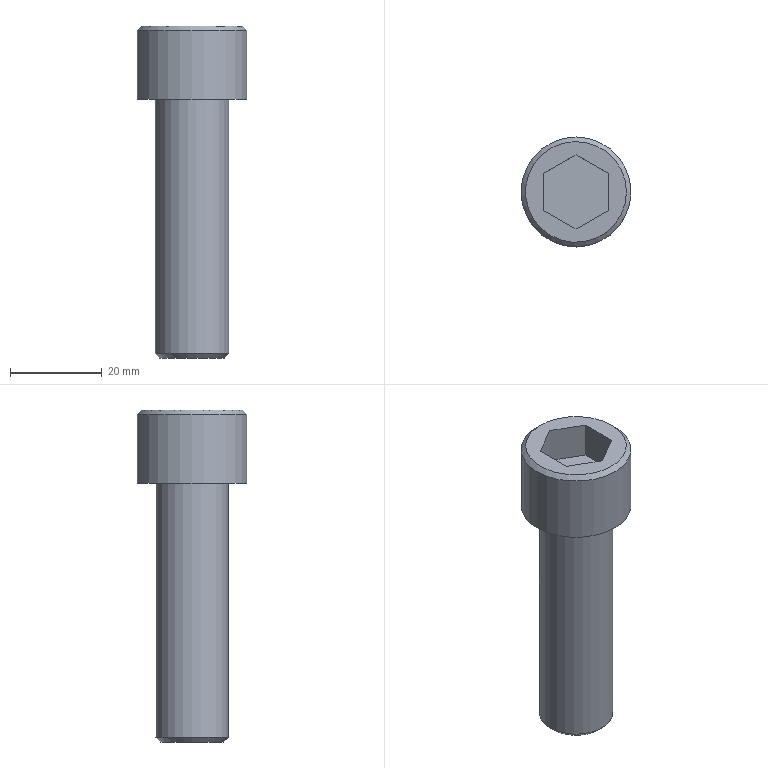Part | STEP file | M16.00-45.00 | 1 solid | 14 faces | box 24 x 24 x 72.5 mm | volume 17180 mm3 | plane 10 | cylinder 2 | cone 2 | commonest cylinder face diameters 16 x1 24 x1